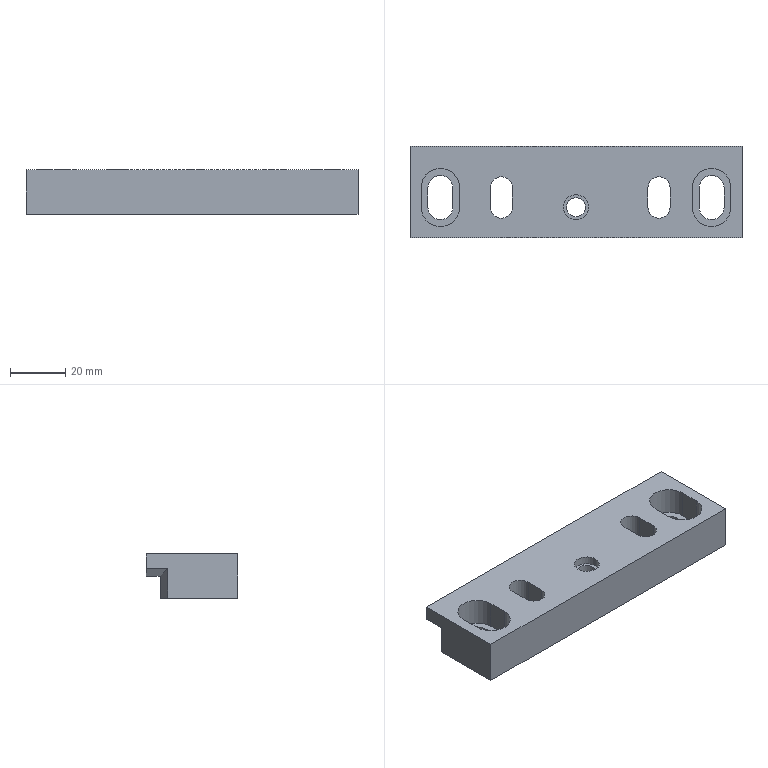Part | STEP file | lll_id4706_x_t | 1 solid | 41 faces | box 120 x 33 x 16 mm | volume 47542 mm3 | plane 27 | cylinder 14 | commonest cylinder face diameters 9 x5 8 x4 14 x4 6.8 x1
STEP:
#1=CARTESIAN_POINT('',(1165.435,-359.7,16.));
#2=VERTEX_POINT('',#1);
#3=CARTESIAN_POINT('',(1173.435,-359.7,16.));
#4=VERTEX_POINT('',#3);
#5=CARTESIAN_POINT('',(1169.435,-359.7,16.));
#6=DIRECTION('',(0.,0.,1.));
#7=DIRECTION('',(-1.,0.,0.));
#8=AXIS2_PLACEMENT_3D('',#5,#6,#7);
#9=CIRCLE('',#8,4.);
#10=EDGE_CURVE('',#2,#4,#9,.T.);
#11=ORIENTED_EDGE('',*,*,#10,.F.);
#12=CARTESIAN_POINT('',(1165.435,-352.7,16.));
#13=VERTEX_POINT('',#12);
#14=CARTESIAN_POINT('',(1165.435,-370.7,16.));
#15=DIRECTION('',(0.,-1.,0.));
#16=VECTOR('',#15,1.);
#17=LINE('',#14,#16);
#18=EDGE_CURVE('',#13,#2,#17,.T.);
#19=ORIENTED_EDGE('',*,*,#18,.F.);
#20=CARTESIAN_POINT('',(1173.435,-352.7,16.));
#21=VERTEX_POINT('',#20);
#22=CARTESIAN_POINT('',(1169.435,-352.7,16.));
#23=DIRECTION('',(0.,0.,1.));
#24=DIRECTION('',(-1.,0.,0.));
#25=AXIS2_PLACEMENT_3D('',#22,#23,#24);
#26=CIRCLE('',#25,4.);
#27=EDGE_CURVE('',#21,#13,#26,.T.);
#28=ORIENTED_EDGE('',*,*,#27,.F.);
#29=CARTESIAN_POINT('',(1173.435,-370.7,16.));
#30=DIRECTION('',(0.,1.,0.));
#31=VECTOR('',#30,1.);
#32=LINE('',#29,#31);
#33=EDGE_CURVE('',#4,#21,#32,.T.);
#34=ORIENTED_EDGE('',*,*,#33,.F.);
#35=EDGE_LOOP('',(#11,#19,#28,#34));
#36=FACE_BOUND('',#35,.T.);
#37=CARTESIAN_POINT('',(1108.435,-359.7,16.));
#38=VERTEX_POINT('',#37);
#39=CARTESIAN_POINT('',(1108.435,-352.7,16.));
#40=VERTEX_POINT('',#39);
#41=CARTESIAN_POINT('',(1108.435,-370.7,16.));
#42=DIRECTION('',(0.,1.,0.));
#43=VECTOR('',#42,1.);
#44=LINE('',#41,#43);
#45=EDGE_CURVE('',#38,#40,#44,.T.);
#46=ORIENTED_EDGE('',*,*,#45,.T.);
#47=CARTESIAN_POINT('',(1116.435,-352.7,16.));
#48=VERTEX_POINT('',#47);
#49=CARTESIAN_POINT('',(1112.435,-352.7,16.));
#50=DIRECTION('',(0.,0.,-1.));
#51=DIRECTION('',(-1.,0.,0.));
#52=AXIS2_PLACEMENT_3D('',#49,#50,#51);
#53=CIRCLE('',#52,4.);
#54=EDGE_CURVE('',#40,#48,#53,.T.);
#55=ORIENTED_EDGE('',*,*,#54,.T.);
#56=CARTESIAN_POINT('',(1116.435,-359.7,16.));
#57=VERTEX_POINT('',#56);
#58=CARTESIAN_POINT('',(1116.435,-370.7,16.));
#59=DIRECTION('',(0.,-1.,0.));
#60=VECTOR('',#59,1.);
#61=LINE('',#58,#60);
#62=EDGE_CURVE('',#48,#57,#61,.T.);
#63=ORIENTED_EDGE('',*,*,#62,.T.);
#64=CARTESIAN_POINT('',(1112.435,-359.7,16.));
#65=DIRECTION('',(0.,0.,-1.));
#66=DIRECTION('',(-1.,0.,0.));
#67=AXIS2_PLACEMENT_3D('',#64,#65,#66);
#68=CIRCLE('',#67,4.);
#69=EDGE_CURVE('',#57,#38,#68,.T.);
#70=ORIENTED_EDGE('',*,*,#69,.T.);
#71=EDGE_LOOP('',(#46,#55,#63,#70));
#72=FACE_BOUND('',#71,.T.);
#73=CARTESIAN_POINT('',(1079.435,-370.7,16.));
#74=VERTEX_POINT('',#73);
#75=CARTESIAN_POINT('',(1199.435,-370.7,16.));
#76=VERTEX_POINT('',#75);
#77=CARTESIAN_POINT('',(1079.435,-370.7,16.));
#78=DIRECTION('',(1.,0.,0.));
#79=VECTOR('',#78,1.);
#80=LINE('',#77,#79);
#81=EDGE_CURVE('',#74,#76,#80,.T.);
#82=ORIENTED_EDGE('',*,*,#81,.T.);
#83=CARTESIAN_POINT('',(1199.435,-337.7,16.));
#84=VERTEX_POINT('',#83);
#85=CARTESIAN_POINT('',(1199.435,-370.7,16.));
#86=DIRECTION('',(0.,1.,0.));
#87=VECTOR('',#86,1.);
#88=LINE('',#85,#87);
#89=EDGE_CURVE('',#76,#84,#88,.T.);
#90=ORIENTED_EDGE('',*,*,#89,.T.);
#91=CARTESIAN_POINT('',(1079.435,-337.7,16.));
#92=VERTEX_POINT('',#91);
#93=CARTESIAN_POINT('',(1159.435,-337.7,16.));
#94=DIRECTION('',(-1.,0.,0.));
#95=VECTOR('',#94,1.);
#96=LINE('',#93,#95);
#97=EDGE_CURVE('',#84,#92,#96,.T.);
#98=ORIENTED_EDGE('',*,*,#97,.T.);
#99=CARTESIAN_POINT('',(1079.435,-337.7,16.));
#100=DIRECTION('',(0.,-1.,0.));
#101=VECTOR('',#100,1.);
#102=LINE('',#99,#101);
#103=EDGE_CURVE('',#92,#74,#102,.T.);
#104=ORIENTED_EDGE('',*,*,#103,.T.);
#105=EDGE_LOOP('',(#82,#90,#98,#104));
#106=FACE_BOUND('',#105,.T.);
#107=CARTESIAN_POINT('',(1083.435,-359.7,16.));
#108=VERTEX_POINT('',#107);
#109=CARTESIAN_POINT('',(1097.435,-359.7,16.));
#110=VERTEX_POINT('',#109);
#111=CARTESIAN_POINT('',(1090.435,-359.7,16.));
#112=DIRECTION('',(0.,0.,1.));
#113=DIRECTION('',(-1.,0.,0.));
#114=AXIS2_PLACEMENT_3D('',#111,#112,#113);
#115=CIRCLE('',#114,7.);
#116=EDGE_CURVE('',#108,#110,#115,.T.);
#117=ORIENTED_EDGE('',*,*,#116,.F.);
#118=CARTESIAN_POINT('',(1083.435,-352.7,16.));
#119=VERTEX_POINT('',#118);
#120=CARTESIAN_POINT('',(1083.435,-370.7,16.));
#121=DIRECTION('',(0.,-1.,0.));
#122=VECTOR('',#121,1.);
#123=LINE('',#120,#122);
#124=EDGE_CURVE('',#119,#108,#123,.T.);
#125=ORIENTED_EDGE('',*,*,#124,.F.);
#126=CARTESIAN_POINT('',(1097.435,-352.7,16.));
#127=VERTEX_POINT('',#126);
#128=CARTESIAN_POINT('',(1090.435,-352.7,16.));
#129=DIRECTION('',(0.,0.,1.));
#130=DIRECTION('',(-1.,0.,0.));
#131=AXIS2_PLACEMENT_3D('',#128,#129,#130);
#132=CIRCLE('',#131,7.);
#133=EDGE_CURVE('',#127,#119,#132,.T.);
#134=ORIENTED_EDGE('',*,*,#133,.F.);
#135=CARTESIAN_POINT('',(1097.435,-370.7,16.));
#136=DIRECTION('',(0.,1.,0.));
#137=VECTOR('',#136,1.);
#138=LINE('',#135,#137);
#139=EDGE_CURVE('',#110,#127,#138,.T.);
#140=ORIENTED_EDGE('',*,*,#139,.F.);
#141=EDGE_LOOP('',(#117,#125,#134,#140));
#142=FACE_BOUND('',#141,.T.);
#143=CARTESIAN_POINT('',(1195.435,-352.7,16.));
#144=VERTEX_POINT('',#143);
#145=CARTESIAN_POINT('',(1181.435,-352.7,16.));
#146=VERTEX_POINT('',#145);
#147=CARTESIAN_POINT('',(1188.435,-352.7,16.));
#148=DIRECTION('',(0.,0.,1.));
#149=DIRECTION('',(-1.,0.,0.));
#150=AXIS2_PLACEMENT_3D('',#147,#148,#149);
#151=CIRCLE('',#150,7.);
#152=EDGE_CURVE('',#144,#146,#151,.T.);
#153=ORIENTED_EDGE('',*,*,#152,.F.);
#154=CARTESIAN_POINT('',(1195.435,-359.7,16.));
#155=VERTEX_POINT('',#154);
#156=CARTESIAN_POINT('',(1195.435,-370.7,16.));
#157=DIRECTION('',(0.,1.,0.));
#158=VECTOR('',#157,1.);
#159=LINE('',#156,#158);
#160=EDGE_CURVE('',#155,#144,#159,.T.);
#161=ORIENTED_EDGE('',*,*,#160,.F.);
#162=CARTESIAN_POINT('',(1181.435,-359.7,16.));
#163=VERTEX_POINT('',#162);
#164=CARTESIAN_POINT('',(1188.435,-359.7,16.));
#165=DIRECTION('',(0.,0.,1.));
#166=DIRECTION('',(-1.,0.,0.));
#167=AXIS2_PLACEMENT_3D('',#164,#165,#166);
#168=CIRCLE('',#167,7.);
#169=EDGE_CURVE('',#163,#155,#168,.T.);
#170=ORIENTED_EDGE('',*,*,#169,.F.);
#171=CARTESIAN_POINT('',(1181.435,-370.7,16.));
#172=DIRECTION('',(0.,-1.,0.));
#173=VECTOR('',#172,1.);
#174=LINE('',#171,#173);
#175=EDGE_CURVE('',#146,#163,#174,.T.);
#176=ORIENTED_EDGE('',*,*,#175,.F.);
#177=EDGE_LOOP('',(#153,#161,#170,#176));
#178=FACE_BOUND('',#177,.T.);
#179=CARTESIAN_POINT('',(1134.935,-359.7,16.));
#180=VERTEX_POINT('',#179);
#181=CARTESIAN_POINT('',(1139.435,-359.7,16.));
#182=DIRECTION('',(0.,0.,1.));
#183=DIRECTION('',(-1.,0.,0.));
#184=AXIS2_PLACEMENT_3D('',#181,#182,#183);
#185=CIRCLE('',#184,4.5);
#186=EDGE_CURVE('',#180,#180,#185,.T.);
#187=ORIENTED_EDGE('',*,*,#186,.F.);
#188=EDGE_LOOP('',(#187));
#189=FACE_BOUND('',#188,.T.);
#190=CARTESIAN_POINT('',(1159.435,-370.7,16.));
#191=DIRECTION('',(0.,0.,1.));
#192=DIRECTION('',(-1.,0.,0.));
#193=AXIS2_PLACEMENT_3D('',#190,#191,#192);
#194=PLANE('',#193);
#195=ADVANCED_FACE('',(#36,#72,#106,#142,#178,#189),#194,.T.);
#196=CARTESIAN_POINT('',(1094.935,-352.7,0.));
#197=VERTEX_POINT('',#196);
#198=CARTESIAN_POINT('',(1094.935,-359.7,0.));
#199=VERTEX_POINT('',#198);
#200=CARTESIAN_POINT('',(1094.935,-352.7,0.));
#201=DIRECTION('',(0.,-1.,0.));
#202=VECTOR('',#201,1.);
#203=LINE('',#200,#202);
#204=EDGE_CURVE('',#197,#199,#203,.T.);
#205=ORIENTED_EDGE('',*,*,#204,.F.);
#206=CARTESIAN_POINT('',(1085.935,-352.7,0.));
#207=VERTEX_POINT('',#206);
#208=CARTESIAN_POINT('',(1090.435,-352.7,0.));
#209=DIRECTION('',(0.,0.,-1.));
#210=DIRECTION('',(-1.,0.,0.));
#211=AXIS2_PLACEMENT_3D('',#208,#209,#210);
#212=CIRCLE('',#211,4.5);
#213=EDGE_CURVE('',#207,#197,#212,.T.);
#214=ORIENTED_EDGE('',*,*,#213,.F.);
#215=CARTESIAN_POINT('',(1085.935,-359.7,0.));
#216=VERTEX_POINT('',#215);
#217=CARTESIAN_POINT('',(1085.935,-359.7,0.));
#218=DIRECTION('',(0.,1.,0.));
#219=VECTOR('',#218,1.);
#220=LINE('',#217,#219);
#221=EDGE_CURVE('',#216,#207,#220,.T.);
#222=ORIENTED_EDGE('',*,*,#221,.F.);
#223=CARTESIAN_POINT('',(1090.435,-359.7,0.));
#224=DIRECTION('',(0.,0.,-1.));
#225=DIRECTION('',(-1.,0.,0.));
#226=AXIS2_PLACEMENT_3D('',#223,#224,#225);
#227=CIRCLE('',#226,4.5);
#228=EDGE_CURVE('',#199,#216,#227,.T.);
#229=ORIENTED_EDGE('',*,*,#228,.F.);
#230=EDGE_LOOP('',(#205,#214,#222,#229));
#231=FACE_BOUND('',#230,.T.);
#232=CARTESIAN_POINT('',(1183.935,-352.7,0.));
#233=VERTEX_POINT('',#232);
#234=CARTESIAN_POINT('',(1183.935,-359.7,0.));
#235=VERTEX_POINT('',#234);
#236=CARTESIAN_POINT('',(1183.935,-352.7,0.));
#237=DIRECTION('',(0.,-1.,0.));
#238=VECTOR('',#237,1.);
#239=LINE('',#236,#238);
#240=EDGE_CURVE('',#233,#235,#239,.T.);
#241=ORIENTED_EDGE('',*,*,#240,.T.);
#242=CARTESIAN_POINT('',(1192.935,-359.7,0.));
#243=VERTEX_POINT('',#242);
#244=CARTESIAN_POINT('',(1188.435,-359.7,0.));
#245=DIRECTION('',(0.,0.,1.));
#246=DIRECTION('',(-1.,0.,0.));
#247=AXIS2_PLACEMENT_3D('',#244,#245,#246);
#248=CIRCLE('',#247,4.5);
#249=EDGE_CURVE('',#235,#243,#248,.T.);
#250=ORIENTED_EDGE('',*,*,#249,.T.);
#251=CARTESIAN_POINT('',(1192.935,-352.7,0.));
#252=VERTEX_POINT('',#251);
#253=CARTESIAN_POINT('',(1192.935,-359.7,0.));
#254=DIRECTION('',(0.,1.,0.));
#255=VECTOR('',#254,1.);
#256=LINE('',#253,#255);
#257=EDGE_CURVE('',#243,#252,#256,.T.);
#258=ORIENTED_EDGE('',*,*,#257,.T.);
#259=CARTESIAN_POINT('',(1188.435,-352.7,0.));
#260=DIRECTION('',(0.,0.,1.));
#261=DIRECTION('',(-1.,0.,0.));
#262=AXIS2_PLACEMENT_3D('',#259,#260,#261);
#263=CIRCLE('',#262,4.5);
#264=EDGE_CURVE('',#252,#233,#263,.T.);
#265=ORIENTED_EDGE('',*,*,#264,.T.);
#266=EDGE_LOOP('',(#241,#250,#258,#265));
#267=FACE_BOUND('',#266,.T.);
#268=CARTESIAN_POINT('',(1199.435,-345.38,0.));
#269=VERTEX_POINT('',#268);
#270=CARTESIAN_POINT('',(1189.434,-342.7,0.));
#271=VERTEX_POINT('',#270);
#272=CARTESIAN_POINT('',(1199.435,-345.38,0.));
#273=DIRECTION('',(-0.9659,0.2588,0.));
#274=VECTOR('',#273,1.);
#275=LINE('',#272,#274);
#276=EDGE_CURVE('',#269,#271,#275,.T.);
#277=ORIENTED_EDGE('',*,*,#276,.F.);
#278=CARTESIAN_POINT('',(1199.435,-370.7,0.));
#279=VERTEX_POINT('',#278);
#280=CARTESIAN_POINT('',(1199.435,-370.7,0.));
#281=DIRECTION('',(0.,1.,0.));
#282=VECTOR('',#281,1.);
#283=LINE('',#280,#282);
#284=EDGE_CURVE('',#279,#269,#283,.T.);
#285=ORIENTED_EDGE('',*,*,#284,.F.);
#286=CARTESIAN_POINT('',(1079.435,-370.7,0.));
#287=VERTEX_POINT('',#286);
#288=CARTESIAN_POINT('',(1079.435,-370.7,0.));
#289=DIRECTION('',(1.,0.,0.));
#290=VECTOR('',#289,1.);
#291=LINE('',#288,#290);
#292=EDGE_CURVE('',#287,#279,#291,.T.);
#293=ORIENTED_EDGE('',*,*,#292,.F.);
#294=CARTESIAN_POINT('',(1079.435,-345.379,0.));
#295=VERTEX_POINT('',#294);
#296=CARTESIAN_POINT('',(1079.435,-337.7,0.));
#297=DIRECTION('',(0.,-1.,0.));
#298=VECTOR('',#297,1.);
#299=LINE('',#296,#298);
#300=EDGE_CURVE('',#295,#287,#299,.T.);
#301=ORIENTED_EDGE('',*,*,#300,.F.);
#302=CARTESIAN_POINT('',(1089.434,-342.7,0.));
#303=VERTEX_POINT('',#302);
#304=CARTESIAN_POINT('',(1089.434,-342.7,0.));
#305=DIRECTION('',(-0.9659,-0.2588,0.));
#306=VECTOR('',#305,1.);
#307=LINE('',#304,#306);
#308=EDGE_CURVE('',#303,#295,#307,.T.);
#309=ORIENTED_EDGE('',*,*,#308,.F.);
#310=CARTESIAN_POINT('',(1149.434,-342.7,0.));
#311=DIRECTION('',(-1.,0.,0.));
#312=VECTOR('',#311,1.);
#313=LINE('',#310,#312);
#314=EDGE_CURVE('',#271,#303,#313,.T.);
#315=ORIENTED_EDGE('',*,*,#314,.F.);
#316=EDGE_LOOP('',(#277,#285,#293,#301,#309,#315));
#317=FACE_BOUND('',#316,.T.);
#318=CARTESIAN_POINT('',(1116.435,-352.7,0.));
#319=VERTEX_POINT('',#318);
#320=CARTESIAN_POINT('',(1108.435,-352.7,0.));
#321=VERTEX_POINT('',#320);
#322=CARTESIAN_POINT('',(1112.435,-352.7,0.));
#323=DIRECTION('',(0.,0.,1.));
#324=DIRECTION('',(-1.,0.,0.));
#325=AXIS2_PLACEMENT_3D('',#322,#323,#324);
#326=CIRCLE('',#325,4.);
#327=EDGE_CURVE('',#319,#321,#326,.T.);
#328=ORIENTED_EDGE('',*,*,#327,.T.);
#329=CARTESIAN_POINT('',(1108.435,-359.7,0.));
#330=VERTEX_POINT('',#329);
#331=CARTESIAN_POINT('',(1108.435,-352.7,0.));
#332=DIRECTION('',(0.,-1.,0.));
#333=VECTOR('',#332,1.);
#334=LINE('',#331,#333);
#335=EDGE_CURVE('',#321,#330,#334,.T.);
#336=ORIENTED_EDGE('',*,*,#335,.T.);
#337=CARTESIAN_POINT('',(1116.435,-359.7,0.));
#338=VERTEX_POINT('',#337);
#339=CARTESIAN_POINT('',(1112.435,-359.7,0.));
#340=DIRECTION('',(0.,0.,1.));
#341=DIRECTION('',(-1.,0.,0.));
#342=AXIS2_PLACEMENT_3D('',#339,#340,#341);
#343=CIRCLE('',#342,4.);
#344=EDGE_CURVE('',#330,#338,#343,.T.);
#345=ORIENTED_EDGE('',*,*,#344,.T.);
#346=CARTESIAN_POINT('',(1116.435,-359.7,0.));
#347=DIRECTION('',(0.,1.,0.));
#348=VECTOR('',#347,1.);
#349=LINE('',#346,#348);
#350=EDGE_CURVE('',#338,#319,#349,.T.);
#351=ORIENTED_EDGE('',*,*,#350,.T.);
#352=EDGE_LOOP('',(#328,#336,#345,#351));
#353=FACE_BOUND('',#352,.T.);
#354=CARTESIAN_POINT('',(1165.435,-359.7,0.));
#355=VERTEX_POINT('',#354);
#356=CARTESIAN_POINT('',(1165.435,-352.7,0.));
#357=VERTEX_POINT('',#356);
#358=CARTESIAN_POINT('',(1165.435,-359.7,0.));
#359=DIRECTION('',(0.,1.,0.));
#360=VECTOR('',#359,1.);
#361=LINE('',#358,#360);
#362=EDGE_CURVE('',#355,#357,#361,.T.);
#363=ORIENTED_EDGE('',*,*,#362,.F.);
#364=CARTESIAN_POINT('',(1173.435,-359.7,0.));
#365=VERTEX_POINT('',#364);
#366=CARTESIAN_POINT('',(1169.435,-359.7,0.));
#367=DIRECTION('',(0.,0.,-1.));
#368=DIRECTION('',(-1.,0.,0.));
#369=AXIS2_PLACEMENT_3D('',#366,#367,#368);
#370=CIRCLE('',#369,4.);
#371=EDGE_CURVE('',#365,#355,#370,.T.);
#372=ORIENTED_EDGE('',*,*,#371,.F.);
#373=CARTESIAN_POINT('',(1173.435,-352.7,0.));
#374=VERTEX_POINT('',#373);
#375=CARTESIAN_POINT('',(1173.435,-352.7,0.));
#376=DIRECTION('',(0.,-1.,0.));
#377=VECTOR('',#376,1.);
#378=LINE('',#375,#377);
#379=EDGE_CURVE('',#374,#365,#378,.T.);
#380=ORIENTED_EDGE('',*,*,#379,.F.);
#381=CARTESIAN_POINT('',(1169.435,-352.7,0.));
#382=DIRECTION('',(0.,0.,-1.));
#383=DIRECTION('',(-1.,0.,0.));
#384=AXIS2_PLACEMENT_3D('',#381,#382,#383);
#385=CIRCLE('',#384,4.);
#386=EDGE_CURVE('',#357,#374,#385,.T.);
#387=ORIENTED_EDGE('',*,*,#386,.F.);
#388=EDGE_LOOP('',(#363,#372,#380,#387));
#389=FACE_BOUND('',#388,.T.);
#390=CARTESIAN_POINT('',(1136.035,-359.7,0.));
#391=VERTEX_POINT('',#390);
#392=CARTESIAN_POINT('',(1139.435,-359.7,0.));
#393=DIRECTION('',(0.,0.,1.));
#394=DIRECTION('',(-1.,0.,0.));
#395=AXIS2_PLACEMENT_3D('',#392,#393,#394);
#396=CIRCLE('',#395,3.4);
#397=EDGE_CURVE('',#391,#391,#396,.T.);
#398=ORIENTED_EDGE('',*,*,#397,.T.);
#399=EDGE_LOOP('',(#398));
#400=FACE_BOUND('',#399,.T.);
#401=CARTESIAN_POINT('',(1159.435,-370.7,0.));
#402=DIRECTION('',(0.,0.,1.));
#403=DIRECTION('',(-1.,0.,0.));
#404=AXIS2_PLACEMENT_3D('',#401,#402,#403);
#405=PLANE('',#404);
#406=ADVANCED_FACE('',(#231,#267,#317,#353,#389,#400),#405,.F.);
#407=CARTESIAN_POINT('',(1199.435,-337.7,10.679));
#408=VERTEX_POINT('',#407);
#409=CARTESIAN_POINT('',(1199.435,-337.7,16.));
#410=DIRECTION('',(0.,0.,-1.));
#411=VECTOR('',#410,1.);
#412=LINE('',#409,#411);
#413=EDGE_CURVE('',#84,#408,#412,.T.);
#414=ORIENTED_EDGE('',*,*,#413,.T.);
#415=CARTESIAN_POINT('',(1189.435,-337.7,8.));
#416=VERTEX_POINT('',#415);
#417=CARTESIAN_POINT('',(1189.435,-337.7,8.));
#418=DIRECTION('',(-0.9659,0.,-0.2588));
#419=VECTOR('',#418,1.);
#420=LINE('',#417,#419);
#421=EDGE_CURVE('',#408,#416,#420,.T.);
#422=ORIENTED_EDGE('',*,*,#421,.T.);
#423=CARTESIAN_POINT('',(1089.435,-337.7,8.));
#424=VERTEX_POINT('',#423);
#425=CARTESIAN_POINT('',(1159.435,-337.7,8.));
#426=DIRECTION('',(1.,0.,0.));
#427=VECTOR('',#426,1.);
#428=LINE('',#425,#427);
#429=EDGE_CURVE('',#424,#416,#428,.T.);
#430=ORIENTED_EDGE('',*,*,#429,.F.);
#431=CARTESIAN_POINT('',(1079.435,-337.7,10.679));
#432=VERTEX_POINT('',#431);
#433=CARTESIAN_POINT('',(1089.435,-337.7,8.));
#434=DIRECTION('',(-0.9659,0.,0.2588));
#435=VECTOR('',#434,1.);
#436=LINE('',#433,#435);
#437=EDGE_CURVE('',#424,#432,#436,.T.);
#438=ORIENTED_EDGE('',*,*,#437,.T.);
#439=CARTESIAN_POINT('',(1079.435,-337.7,16.));
#440=DIRECTION('',(0.,0.,-1.));
#441=VECTOR('',#440,1.);
#442=LINE('',#439,#441);
#443=EDGE_CURVE('',#92,#432,#442,.T.);
#444=ORIENTED_EDGE('',*,*,#443,.F.);
#445=ORIENTED_EDGE('',*,*,#97,.F.);
#446=EDGE_LOOP('',(#414,#422,#430,#438,#444,#445));
#447=FACE_OUTER_BOUND('',#446,.T.);
#448=CARTESIAN_POINT('',(1159.435,-337.7,16.));
#449=DIRECTION('',(0.,-1.,0.));
#450=DIRECTION('',(0.,0.,1.));
#451=AXIS2_PLACEMENT_3D('',#448,#449,#450);
#452=PLANE('',#451);
#453=ADVANCED_FACE('',(#447),#452,.F.);
#454=ORIENTED_EDGE('',*,*,#292,.T.);
#455=CARTESIAN_POINT('',(1199.435,-370.7,16.));
#456=DIRECTION('',(0.,0.,-1.));
#457=VECTOR('',#456,1.);
#458=LINE('',#455,#457);
#459=EDGE_CURVE('',#76,#279,#458,.T.);
#460=ORIENTED_EDGE('',*,*,#459,.F.);
#461=ORIENTED_EDGE('',*,*,#81,.F.);
#462=CARTESIAN_POINT('',(1079.435,-370.7,16.));
#463=DIRECTION('',(0.,0.,-1.));
#464=VECTOR('',#463,1.);
#465=LINE('',#462,#464);
#466=EDGE_CURVE('',#74,#287,#465,.T.);
#467=ORIENTED_EDGE('',*,*,#466,.T.);
#468=EDGE_LOOP('',(#454,#460,#461,#467));
#469=FACE_OUTER_BOUND('',#468,.T.);
#470=CARTESIAN_POINT('',(1079.435,-370.7,16.));
#471=DIRECTION('',(0.,1.,0.));
#472=DIRECTION('',(0.,0.,-1.));
#473=AXIS2_PLACEMENT_3D('',#470,#471,#472);
#474=PLANE('',#473);
#475=ADVANCED_FACE('',(#469),#474,.F.);
#476=CARTESIAN_POINT('',(1199.435,-345.38,10.679));
#477=VERTEX_POINT('',#476);
#478=CARTESIAN_POINT('',(1199.435,-345.38,8.));
#479=DIRECTION('',(0.,0.,-1.));
#480=VECTOR('',#479,1.);
#481=LINE('',#478,#480);
#482=EDGE_CURVE('',#477,#269,#481,.T.);
#483=ORIENTED_EDGE('',*,*,#482,.F.);
#484=CARTESIAN_POINT('',(1199.435,-337.7,10.679));
#485=DIRECTION('',(0.,1.,0.));
#486=VECTOR('',#485,1.);
#487=LINE('',#484,#486);
#488=EDGE_CURVE('',#477,#408,#487,.T.);
#489=ORIENTED_EDGE('',*,*,#488,.T.);
#490=ORIENTED_EDGE('',*,*,#413,.F.);
#491=ORIENTED_EDGE('',*,*,#89,.F.);
#492=ORIENTED_EDGE('',*,*,#459,.T.);
#493=ORIENTED_EDGE('',*,*,#284,.T.);
#494=EDGE_LOOP('',(#483,#489,#490,#491,#492,#493));
#495=FACE_OUTER_BOUND('',#494,.T.);
#496=CARTESIAN_POINT('',(1199.435,-370.7,16.));
#497=DIRECTION('',(-1.,0.,0.));
#498=DIRECTION('',(0.,0.,-1.));
#499=AXIS2_PLACEMENT_3D('',#496,#497,#498);
#500=PLANE('',#499);
#501=ADVANCED_FACE('',(#495),#500,.F.);
#502=ORIENTED_EDGE('',*,*,#443,.T.);
#503=CARTESIAN_POINT('',(1079.435,-345.379,10.679));
#504=VERTEX_POINT('',#503);
#505=CARTESIAN_POINT('',(1079.435,-345.379,10.679));
#506=DIRECTION('',(0.,-1.,0.));
#507=VECTOR('',#506,1.);
#508=LINE('',#505,#507);
#509=EDGE_CURVE('',#432,#504,#508,.T.);
#510=ORIENTED_EDGE('',*,*,#509,.T.);
#511=CARTESIAN_POINT('',(1079.435,-345.379,8.));
#512=DIRECTION('',(0.,0.,-1.));
#513=VECTOR('',#512,1.);
#514=LINE('',#511,#513);
#515=EDGE_CURVE('',#504,#295,#514,.T.);
#516=ORIENTED_EDGE('',*,*,#515,.T.);
#517=ORIENTED_EDGE('',*,*,#300,.T.);
#518=ORIENTED_EDGE('',*,*,#466,.F.);
#519=ORIENTED_EDGE('',*,*,#103,.F.);
#520=EDGE_LOOP('',(#502,#510,#516,#517,#518,#519));
#521=FACE_OUTER_BOUND('',#520,.T.);
#522=CARTESIAN_POINT('',(1079.435,-337.7,16.));
#523=DIRECTION('',(1.,0.,0.));
#524=DIRECTION('',(0.,0.,1.));
#525=AXIS2_PLACEMENT_3D('',#522,#523,#524);
#526=PLANE('',#525);
#527=ADVANCED_FACE('',(#521),#526,.F.);
#528=ORIENTED_EDGE('',*,*,#429,.T.);
#529=CARTESIAN_POINT('',(1189.435,-342.701,8.));
#530=VERTEX_POINT('',#529);
#531=CARTESIAN_POINT('',(1189.435,-345.38,8.));
#532=DIRECTION('',(0.,-1.,0.));
#533=VECTOR('',#532,1.);
#534=LINE('',#531,#533);
#535=EDGE_CURVE('',#416,#530,#534,.T.);
#536=ORIENTED_EDGE('',*,*,#535,.T.);
#537=CARTESIAN_POINT('',(1189.434,-342.7,8.));
#538=VERTEX_POINT('',#537);
#539=CARTESIAN_POINT('',(1199.435,-345.38,8.));
#540=DIRECTION('',(0.9659,-0.2588,0.));
#541=VECTOR('',#540,1.);
#542=LINE('',#539,#541);
#543=EDGE_CURVE('',#538,#530,#542,.T.);
#544=ORIENTED_EDGE('',*,*,#543,.F.);
#545=CARTESIAN_POINT('',(1089.435,-342.7,8.));
#546=VERTEX_POINT('',#545);
#547=CARTESIAN_POINT('',(1149.434,-342.7,8.));
#548=DIRECTION('',(1.,0.,0.));
#549=VECTOR('',#548,1.);
#550=LINE('',#547,#549);
#551=EDGE_CURVE('',#546,#538,#550,.T.);
#552=ORIENTED_EDGE('',*,*,#551,.F.);
#553=CARTESIAN_POINT('',(1089.435,-337.7,8.));
#554=DIRECTION('',(0.,1.,0.));
#555=VECTOR('',#554,1.);
#556=LINE('',#553,#555);
#557=EDGE_CURVE('',#546,#424,#556,.T.);
#558=ORIENTED_EDGE('',*,*,#557,.T.);
#559=EDGE_LOOP('',(#528,#536,#544,#552,#558));
#560=FACE_OUTER_BOUND('',#559,.T.);
#561=CARTESIAN_POINT('',(1181.706,-317.091,8.));
#562=DIRECTION('',(0.,0.,-1.));
#563=DIRECTION('',(1.,0.,0.));
#564=AXIS2_PLACEMENT_3D('',#561,#562,#563);
#565=PLANE('',#564);
#566=ADVANCED_FACE('',(#560),#565,.T.);
#567=ORIENTED_EDGE('',*,*,#276,.T.);
#568=CARTESIAN_POINT('',(1189.434,-342.7,8.));
#569=DIRECTION('',(0.,0.,1.));
#570=VECTOR('',#569,1.);
#571=LINE('',#568,#570);
#572=EDGE_CURVE('',#271,#538,#571,.T.);
#573=ORIENTED_EDGE('',*,*,#572,.T.);
#574=ORIENTED_EDGE('',*,*,#543,.T.);
#575=CARTESIAN_POINT('',(1198.807,-345.212,10.511));
#576=DIRECTION('',(0.9351,-0.2506,0.2506));
#577=VECTOR('',#576,1.);
#578=LINE('',#575,#577);
#579=EDGE_CURVE('',#530,#477,#578,.T.);
#580=ORIENTED_EDGE('',*,*,#579,.T.);
#581=ORIENTED_EDGE('',*,*,#482,.T.);
#582=EDGE_LOOP('',(#567,#573,#574,#580,#581));
#583=FACE_OUTER_BOUND('',#582,.T.);
#584=CARTESIAN_POINT('',(1199.435,-345.38,8.));
#585=DIRECTION('',(-0.2588,-0.9659,0.));
#586=DIRECTION('',(0.9659,-0.2588,0.));
#587=AXIS2_PLACEMENT_3D('',#584,#585,#586);
#588=PLANE('',#587);
#589=ADVANCED_FACE('',(#583),#588,.F.);
#590=ORIENTED_EDGE('',*,*,#314,.T.);
#591=CARTESIAN_POINT('',(1089.434,-342.7,8.));
#592=VERTEX_POINT('',#591);
#593=CARTESIAN_POINT('',(1089.434,-342.7,8.));
#594=DIRECTION('',(0.,0.,1.));
#595=VECTOR('',#594,1.);
#596=LINE('',#593,#595);
#597=EDGE_CURVE('',#303,#592,#596,.T.);
#598=ORIENTED_EDGE('',*,*,#597,.T.);
#599=CARTESIAN_POINT('',(1145.414,-342.7,-7.));
#600=DIRECTION('',(0.9659,0.,-0.2588));
#601=VECTOR('',#600,1.);
#602=LINE('',#599,#601);
#603=EDGE_CURVE('',#592,#546,#602,.T.);
#604=ORIENTED_EDGE('',*,*,#603,.T.);
#605=ORIENTED_EDGE('',*,*,#551,.T.);
#606=ORIENTED_EDGE('',*,*,#572,.F.);
#607=EDGE_LOOP('',(#590,#598,#604,#605,#606));
#608=FACE_OUTER_BOUND('',#607,.T.);
#609=CARTESIAN_POINT('',(1149.434,-342.7,8.));
#610=DIRECTION('',(0.,-1.,0.));
#611=DIRECTION('',(0.,0.,1.));
#612=AXIS2_PLACEMENT_3D('',#609,#610,#611);
#613=PLANE('',#612);
#614=ADVANCED_FACE('',(#608),#613,.F.);
#615=ORIENTED_EDGE('',*,*,#308,.T.);
#616=ORIENTED_EDGE('',*,*,#515,.F.);
#617=CARTESIAN_POINT('',(1089.434,-342.7,8.));
#618=DIRECTION('',(0.9351,0.2506,-0.2506));
#619=VECTOR('',#618,1.);
#620=LINE('',#617,#619);
#621=EDGE_CURVE('',#504,#592,#620,.T.);
#622=ORIENTED_EDGE('',*,*,#621,.T.);
#623=ORIENTED_EDGE('',*,*,#597,.F.);
#624=EDGE_LOOP('',(#615,#616,#622,#623));
#625=FACE_OUTER_BOUND('',#624,.T.);
#626=CARTESIAN_POINT('',(1089.434,-342.7,8.));
#627=DIRECTION('',(0.2588,-0.9659,0.));
#628=DIRECTION('',(0.9659,0.2588,0.));
#629=AXIS2_PLACEMENT_3D('',#626,#627,#628);
#630=PLANE('',#629);
#631=ADVANCED_FACE('',(#625),#630,.F.);
#632=CARTESIAN_POINT('',(1108.435,-352.7,47.));
#633=DIRECTION('',(0.,0.,1.));
#634=VECTOR('',#633,1.);
#635=LINE('',#632,#634);
#636=EDGE_CURVE('',#321,#40,#635,.T.);
#637=ORIENTED_EDGE('',*,*,#636,.F.);
#638=ORIENTED_EDGE('',*,*,#327,.F.);
#639=CARTESIAN_POINT('',(1116.435,-352.7,47.));
#640=DIRECTION('',(0.,0.,1.));
#641=VECTOR('',#640,1.);
#642=LINE('',#639,#641);
#643=EDGE_CURVE('',#319,#48,#642,.T.);
#644=ORIENTED_EDGE('',*,*,#643,.T.);
#645=ORIENTED_EDGE('',*,*,#54,.F.);
#646=EDGE_LOOP('',(#637,#638,#644,#645));
#647=FACE_OUTER_BOUND('',#646,.T.);
#648=CARTESIAN_POINT('',(1112.435,-352.7,47.));
#649=DIRECTION('',(0.,0.,-1.));
#650=DIRECTION('',(1.,0.,0.));
#651=AXIS2_PLACEMENT_3D('',#648,#649,#650);
#652=CYLINDRICAL_SURFACE('',#651,4.);
#653=ADVANCED_FACE('',(#647),#652,.F.);
#654=CARTESIAN_POINT('',(1108.435,-359.7,47.));
#655=DIRECTION('',(0.,0.,1.));
#656=VECTOR('',#655,1.);
#657=LINE('',#654,#656);
#658=EDGE_CURVE('',#330,#38,#657,.T.);
#659=ORIENTED_EDGE('',*,*,#658,.F.);
#660=ORIENTED_EDGE('',*,*,#335,.F.);
#661=ORIENTED_EDGE('',*,*,#636,.T.);
#662=ORIENTED_EDGE('',*,*,#45,.F.);
#663=EDGE_LOOP('',(#659,#660,#661,#662));
#664=FACE_OUTER_BOUND('',#663,.T.);
#665=CARTESIAN_POINT('',(1108.435,-352.7,47.));
#666=DIRECTION('',(1.,0.,0.));
#667=DIRECTION('',(0.,0.,1.));
#668=AXIS2_PLACEMENT_3D('',#665,#666,#667);
#669=PLANE('',#668);
#670=ADVANCED_FACE('',(#664),#669,.T.);
#671=CARTESIAN_POINT('',(1116.435,-359.7,47.));
#672=DIRECTION('',(0.,0.,1.));
#673=VECTOR('',#672,1.);
#674=LINE('',#671,#673);
#675=EDGE_CURVE('',#338,#57,#674,.T.);
#676=ORIENTED_EDGE('',*,*,#675,.F.);
#677=ORIENTED_EDGE('',*,*,#344,.F.);
#678=ORIENTED_EDGE('',*,*,#658,.T.);
#679=ORIENTED_EDGE('',*,*,#69,.F.);
#680=EDGE_LOOP('',(#676,#677,#678,#679));
#681=FACE_OUTER_BOUND('',#680,.T.);
#682=CARTESIAN_POINT('',(1112.435,-359.7,47.));
#683=DIRECTION('',(0.,0.,-1.));
#684=DIRECTION('',(1.,0.,0.));
#685=AXIS2_PLACEMENT_3D('',#682,#683,#684);
#686=CYLINDRICAL_SURFACE('',#685,4.);
#687=ADVANCED_FACE('',(#681),#686,.F.);
#688=ORIENTED_EDGE('',*,*,#643,.F.);
#689=ORIENTED_EDGE('',*,*,#350,.F.);
#690=ORIENTED_EDGE('',*,*,#675,.T.);
#691=ORIENTED_EDGE('',*,*,#62,.F.);
#692=EDGE_LOOP('',(#688,#689,#690,#691));
#693=FACE_OUTER_BOUND('',#692,.T.);
#694=CARTESIAN_POINT('',(1116.435,-359.7,47.));
#695=DIRECTION('',(-1.,0.,0.));
#696=DIRECTION('',(0.,0.,-1.));
#697=AXIS2_PLACEMENT_3D('',#694,#695,#696);
#698=PLANE('',#697);
#699=ADVANCED_FACE('',(#693),#698,.T.);
#700=CARTESIAN_POINT('',(1183.935,-359.7,6.));
#701=VERTEX_POINT('',#700);
#702=CARTESIAN_POINT('',(1183.935,-352.7,6.));
#703=VERTEX_POINT('',#702);
#704=CARTESIAN_POINT('',(1183.935,-352.7,6.));
#705=DIRECTION('',(0.,1.,0.));
#706=VECTOR('',#705,1.);
#707=LINE('',#704,#706);
#708=EDGE_CURVE('',#701,#703,#707,.T.);
#709=ORIENTED_EDGE('',*,*,#708,.F.);
#710=CARTESIAN_POINT('',(1183.935,-359.7,47.));
#711=DIRECTION('',(0.,0.,1.));
#712=VECTOR('',#711,1.);
#713=LINE('',#710,#712);
#714=EDGE_CURVE('',#235,#701,#713,.T.);
#715=ORIENTED_EDGE('',*,*,#714,.F.);
#716=ORIENTED_EDGE('',*,*,#240,.F.);
#717=CARTESIAN_POINT('',(1183.935,-352.7,47.));
#718=DIRECTION('',(0.,0.,1.));
#719=VECTOR('',#718,1.);
#720=LINE('',#717,#719);
#721=EDGE_CURVE('',#233,#703,#720,.T.);
#722=ORIENTED_EDGE('',*,*,#721,.T.);
#723=EDGE_LOOP('',(#709,#715,#716,#722));
#724=FACE_OUTER_BOUND('',#723,.T.);
#725=CARTESIAN_POINT('',(1183.935,-352.7,47.));
#726=DIRECTION('',(1.,0.,0.));
#727=DIRECTION('',(0.,0.,1.));
#728=AXIS2_PLACEMENT_3D('',#725,#726,#727);
#729=PLANE('',#728);
#730=ADVANCED_FACE('',(#724),#729,.T.);
#731=CARTESIAN_POINT('',(1192.935,-359.7,6.));
#732=VERTEX_POINT('',#731);
#733=CARTESIAN_POINT('',(1188.435,-359.7,6.));
#734=DIRECTION('',(0.,0.,-1.));
#735=DIRECTION('',(1.,0.,0.));
#736=AXIS2_PLACEMENT_3D('',#733,#734,#735);
#737=CIRCLE('',#736,4.5);
#738=EDGE_CURVE('',#732,#701,#737,.T.);
#739=ORIENTED_EDGE('',*,*,#738,.F.);
#740=CARTESIAN_POINT('',(1192.935,-359.7,47.));
#741=DIRECTION('',(0.,0.,1.));
#742=VECTOR('',#741,1.);
#743=LINE('',#740,#742);
#744=EDGE_CURVE('',#243,#732,#743,.T.);
#745=ORIENTED_EDGE('',*,*,#744,.F.);
#746=ORIENTED_EDGE('',*,*,#249,.F.);
#747=ORIENTED_EDGE('',*,*,#714,.T.);
#748=EDGE_LOOP('',(#739,#745,#746,#747));
#749=FACE_OUTER_BOUND('',#748,.T.);
#750=CARTESIAN_POINT('',(1188.435,-359.7,47.));
#751=DIRECTION('',(0.,0.,-1.));
#752=DIRECTION('',(1.,0.,0.));
#753=AXIS2_PLACEMENT_3D('',#750,#751,#752);
#754=CYLINDRICAL_SURFACE('',#753,4.5);
#755=ADVANCED_FACE('',(#749),#754,.F.);
#756=CARTESIAN_POINT('',(1192.935,-352.7,6.));
#757=VERTEX_POINT('',#756);
#758=CARTESIAN_POINT('',(1192.935,-359.7,6.));
#759=DIRECTION('',(0.,-1.,0.));
#760=VECTOR('',#759,1.);
#761=LINE('',#758,#760);
#762=EDGE_CURVE('',#757,#732,#761,.T.);
#763=ORIENTED_EDGE('',*,*,#762,.F.);
#764=CARTESIAN_POINT('',(1192.935,-352.7,47.));
#765=DIRECTION('',(0.,0.,1.));
#766=VECTOR('',#765,1.);
#767=LINE('',#764,#766);
#768=EDGE_CURVE('',#252,#757,#767,.T.);
#769=ORIENTED_EDGE('',*,*,#768,.F.);
#770=ORIENTED_EDGE('',*,*,#257,.F.);
#771=ORIENTED_EDGE('',*,*,#744,.T.);
#772=EDGE_LOOP('',(#763,#769,#770,#771));
#773=FACE_OUTER_BOUND('',#772,.T.);
#774=CARTESIAN_POINT('',(1192.935,-359.7,47.));
#775=DIRECTION('',(-1.,0.,0.));
#776=DIRECTION('',(0.,0.,-1.));
#777=AXIS2_PLACEMENT_3D('',#774,#775,#776);
#778=PLANE('',#777);
#779=ADVANCED_FACE('',(#773),#778,.T.);
#780=CARTESIAN_POINT('',(1188.435,-352.7,6.));
#781=DIRECTION('',(0.,0.,-1.));
#782=DIRECTION('',(1.,0.,0.));
#783=AXIS2_PLACEMENT_3D('',#780,#781,#782);
#784=CIRCLE('',#783,4.5);
#785=EDGE_CURVE('',#703,#757,#784,.T.);
#786=ORIENTED_EDGE('',*,*,#785,.F.);
#787=ORIENTED_EDGE('',*,*,#721,.F.);
#788=ORIENTED_EDGE('',*,*,#264,.F.);
#789=ORIENTED_EDGE('',*,*,#768,.T.);
#790=EDGE_LOOP('',(#786,#787,#788,#789));
#791=FACE_OUTER_BOUND('',#790,.T.);
#792=CARTESIAN_POINT('',(1188.435,-352.7,47.));
#793=DIRECTION('',(0.,0.,-1.));
#794=DIRECTION('',(1.,0.,0.));
#795=AXIS2_PLACEMENT_3D('',#792,#793,#794);
#796=CYLINDRICAL_SURFACE('',#795,4.5);
#797=ADVANCED_FACE('',(#791),#796,.F.);
#798=ORIENTED_EDGE('',*,*,#10,.T.);
#799=CARTESIAN_POINT('',(1173.435,-359.7,47.));
#800=DIRECTION('',(0.,0.,1.));
#801=VECTOR('',#800,1.);
#802=LINE('',#799,#801);
#803=EDGE_CURVE('',#365,#4,#802,.T.);
#804=ORIENTED_EDGE('',*,*,#803,.F.);
#805=ORIENTED_EDGE('',*,*,#371,.T.);
#806=CARTESIAN_POINT('',(1165.435,-359.7,47.));
#807=DIRECTION('',(0.,0.,1.));
#808=VECTOR('',#807,1.);
#809=LINE('',#806,#808);
#810=EDGE_CURVE('',#355,#2,#809,.T.);
#811=ORIENTED_EDGE('',*,*,#810,.T.);
#812=EDGE_LOOP('',(#798,#804,#805,#811));
#813=FACE_OUTER_BOUND('',#812,.T.);
#814=CARTESIAN_POINT('',(1169.435,-359.7,47.));
#815=DIRECTION('',(0.,0.,-1.));
#816=DIRECTION('',(1.,0.,0.));
#817=AXIS2_PLACEMENT_3D('',#814,#815,#816);
#818=CYLINDRICAL_SURFACE('',#817,4.);
#819=ADVANCED_FACE('',(#813),#818,.F.);
#820=ORIENTED_EDGE('',*,*,#18,.T.);
#821=ORIENTED_EDGE('',*,*,#810,.F.);
#822=ORIENTED_EDGE('',*,*,#362,.T.);
#823=CARTESIAN_POINT('',(1165.435,-352.7,47.));
#824=DIRECTION('',(0.,0.,1.));
#825=VECTOR('',#824,1.);
#826=LINE('',#823,#825);
#827=EDGE_CURVE('',#357,#13,#826,.T.);
#828=ORIENTED_EDGE('',*,*,#827,.T.);
#829=EDGE_LOOP('',(#820,#821,#822,#828));
#830=FACE_OUTER_BOUND('',#829,.T.);
#831=CARTESIAN_POINT('',(1165.435,-359.7,47.));
#832=DIRECTION('',(-1.,0.,0.));
#833=DIRECTION('',(0.,0.,-1.));
#834=AXIS2_PLACEMENT_3D('',#831,#832,#833);
#835=PLANE('',#834);
#836=ADVANCED_FACE('',(#830),#835,.F.);
#837=ORIENTED_EDGE('',*,*,#27,.T.);
#838=ORIENTED_EDGE('',*,*,#827,.F.);
#839=ORIENTED_EDGE('',*,*,#386,.T.);
#840=CARTESIAN_POINT('',(1173.435,-352.7,47.));
#841=DIRECTION('',(0.,0.,1.));
#842=VECTOR('',#841,1.);
#843=LINE('',#840,#842);
#844=EDGE_CURVE('',#374,#21,#843,.T.);
#845=ORIENTED_EDGE('',*,*,#844,.T.);
#846=EDGE_LOOP('',(#837,#838,#839,#845));
#847=FACE_OUTER_BOUND('',#846,.T.);
#848=CARTESIAN_POINT('',(1169.435,-352.7,47.));
#849=DIRECTION('',(0.,0.,-1.));
#850=DIRECTION('',(1.,0.,0.));
#851=AXIS2_PLACEMENT_3D('',#848,#849,#850);
#852=CYLINDRICAL_SURFACE('',#851,4.);
#853=ADVANCED_FACE('',(#847),#852,.F.);
#854=ORIENTED_EDGE('',*,*,#33,.T.);
#855=ORIENTED_EDGE('',*,*,#844,.F.);
#856=ORIENTED_EDGE('',*,*,#379,.T.);
#857=ORIENTED_EDGE('',*,*,#803,.T.);
#858=EDGE_LOOP('',(#854,#855,#856,#857));
#859=FACE_OUTER_BOUND('',#858,.T.);
#860=CARTESIAN_POINT('',(1173.435,-352.7,47.));
#861=DIRECTION('',(1.,0.,0.));
#862=DIRECTION('',(0.,0.,1.));
#863=AXIS2_PLACEMENT_3D('',#860,#861,#862);
#864=PLANE('',#863);
#865=ADVANCED_FACE('',(#859),#864,.F.);
#866=CARTESIAN_POINT('',(1142.835,-359.7,13.));
#867=VERTEX_POINT('',#866);
#868=CARTESIAN_POINT('',(1139.435,-359.7,13.));
#869=DIRECTION('',(0.,0.,-1.));
#870=DIRECTION('',(1.,0.,0.));
#871=AXIS2_PLACEMENT_3D('',#868,#869,#870);
#872=CIRCLE('',#871,3.4);
#873=EDGE_CURVE('',#867,#867,#872,.T.);
#874=ORIENTED_EDGE('',*,*,#873,.F.);
#875=EDGE_LOOP('',(#874));
#876=FACE_BOUND('',#875,.T.);
#877=ORIENTED_EDGE('',*,*,#397,.F.);
#878=EDGE_LOOP('',(#877));
#879=FACE_BOUND('',#878,.T.);
#880=CARTESIAN_POINT('',(1139.435,-359.7,47.));
#881=DIRECTION('',(0.,0.,-1.));
#882=DIRECTION('',(1.,0.,0.));
#883=AXIS2_PLACEMENT_3D('',#880,#881,#882);
#884=CYLINDRICAL_SURFACE('',#883,3.4);
#885=ADVANCED_FACE('',(#876,#879),#884,.F.);
#886=CARTESIAN_POINT('',(1094.935,-352.7,6.));
#887=VERTEX_POINT('',#886);
#888=CARTESIAN_POINT('',(1094.935,-352.7,47.));
#889=DIRECTION('',(0.,0.,1.));
#890=VECTOR('',#889,1.);
#891=LINE('',#888,#890);
#892=EDGE_CURVE('',#197,#887,#891,.T.);
#893=ORIENTED_EDGE('',*,*,#892,.T.);
#894=CARTESIAN_POINT('',(1085.935,-352.7,6.));
#895=VERTEX_POINT('',#894);
#896=CARTESIAN_POINT('',(1090.435,-352.7,6.));
#897=DIRECTION('',(0.,0.,1.));
#898=DIRECTION('',(1.,0.,0.));
#899=AXIS2_PLACEMENT_3D('',#896,#897,#898);
#900=CIRCLE('',#899,4.5);
#901=EDGE_CURVE('',#887,#895,#900,.T.);
#902=ORIENTED_EDGE('',*,*,#901,.T.);
#903=CARTESIAN_POINT('',(1085.935,-352.7,47.));
#904=DIRECTION('',(0.,0.,1.));
#905=VECTOR('',#904,1.);
#906=LINE('',#903,#905);
#907=EDGE_CURVE('',#207,#895,#906,.T.);
#908=ORIENTED_EDGE('',*,*,#907,.F.);
#909=ORIENTED_EDGE('',*,*,#213,.T.);
#910=EDGE_LOOP('',(#893,#902,#908,#909));
#911=FACE_OUTER_BOUND('',#910,.T.);
#912=CARTESIAN_POINT('',(1090.435,-352.7,47.));
#913=DIRECTION('',(0.,0.,-1.));
#914=DIRECTION('',(1.,0.,0.));
#915=AXIS2_PLACEMENT_3D('',#912,#913,#914);
#916=CYLINDRICAL_SURFACE('',#915,4.5);
#917=ADVANCED_FACE('',(#911),#916,.F.);
#918=CARTESIAN_POINT('',(1094.935,-359.7,6.));
#919=VERTEX_POINT('',#918);
#920=CARTESIAN_POINT('',(1094.935,-359.7,47.));
#921=DIRECTION('',(0.,0.,1.));
#922=VECTOR('',#921,1.);
#923=LINE('',#920,#922);
#924=EDGE_CURVE('',#199,#919,#923,.T.);
#925=ORIENTED_EDGE('',*,*,#924,.T.);
#926=CARTESIAN_POINT('',(1094.935,-352.7,6.));
#927=DIRECTION('',(0.,1.,0.));
#928=VECTOR('',#927,1.);
#929=LINE('',#926,#928);
#930=EDGE_CURVE('',#919,#887,#929,.T.);
#931=ORIENTED_EDGE('',*,*,#930,.T.);
#932=ORIENTED_EDGE('',*,*,#892,.F.);
#933=ORIENTED_EDGE('',*,*,#204,.T.);
#934=EDGE_LOOP('',(#925,#931,#932,#933));
#935=FACE_OUTER_BOUND('',#934,.T.);
#936=CARTESIAN_POINT('',(1094.935,-352.7,47.));
#937=DIRECTION('',(1.,0.,0.));
#938=DIRECTION('',(0.,0.,1.));
#939=AXIS2_PLACEMENT_3D('',#936,#937,#938);
#940=PLANE('',#939);
#941=ADVANCED_FACE('',(#935),#940,.F.);
#942=CARTESIAN_POINT('',(1085.935,-359.7,6.));
#943=VERTEX_POINT('',#942);
#944=CARTESIAN_POINT('',(1085.935,-359.7,47.));
#945=DIRECTION('',(0.,0.,1.));
#946=VECTOR('',#945,1.);
#947=LINE('',#944,#946);
#948=EDGE_CURVE('',#216,#943,#947,.T.);
#949=ORIENTED_EDGE('',*,*,#948,.T.);
#950=CARTESIAN_POINT('',(1090.435,-359.7,6.));
#951=DIRECTION('',(0.,0.,1.));
#952=DIRECTION('',(1.,0.,0.));
#953=AXIS2_PLACEMENT_3D('',#950,#951,#952);
#954=CIRCLE('',#953,4.5);
#955=EDGE_CURVE('',#943,#919,#954,.T.);
#956=ORIENTED_EDGE('',*,*,#955,.T.);
#957=ORIENTED_EDGE('',*,*,#924,.F.);
#958=ORIENTED_EDGE('',*,*,#228,.T.);
#959=EDGE_LOOP('',(#949,#956,#957,#958));
#960=FACE_OUTER_BOUND('',#959,.T.);
#961=CARTESIAN_POINT('',(1090.435,-359.7,47.));
#962=DIRECTION('',(0.,0.,-1.));
#963=DIRECTION('',(1.,0.,0.));
#964=AXIS2_PLACEMENT_3D('',#961,#962,#963);
#965=CYLINDRICAL_SURFACE('',#964,4.5);
#966=ADVANCED_FACE('',(#960),#965,.F.);
#967=ORIENTED_EDGE('',*,*,#907,.T.);
#968=CARTESIAN_POINT('',(1085.935,-359.7,6.));
#969=DIRECTION('',(0.,-1.,0.));
#970=VECTOR('',#969,1.);
#971=LINE('',#968,#970);
#972=EDGE_CURVE('',#895,#943,#971,.T.);
#973=ORIENTED_EDGE('',*,*,#972,.T.);
#974=ORIENTED_EDGE('',*,*,#948,.F.);
#975=ORIENTED_EDGE('',*,*,#221,.T.);
#976=EDGE_LOOP('',(#967,#973,#974,#975));
#977=FACE_OUTER_BOUND('',#976,.T.);
#978=CARTESIAN_POINT('',(1085.935,-359.7,47.));
#979=DIRECTION('',(-1.,0.,0.));
#980=DIRECTION('',(0.,0.,-1.));
#981=AXIS2_PLACEMENT_3D('',#978,#979,#980);
#982=PLANE('',#981);
#983=ADVANCED_FACE('',(#977),#982,.F.);
#984=CARTESIAN_POINT('',(1083.435,-359.7,6.));
#985=VERTEX_POINT('',#984);
#986=CARTESIAN_POINT('',(1097.435,-359.7,6.));
#987=VERTEX_POINT('',#986);
#988=CARTESIAN_POINT('',(1090.435,-359.7,6.));
#989=DIRECTION('',(0.,0.,1.));
#990=DIRECTION('',(-1.,0.,0.));
#991=AXIS2_PLACEMENT_3D('',#988,#989,#990);
#992=CIRCLE('',#991,7.);
#993=EDGE_CURVE('',#985,#987,#992,.T.);
#994=ORIENTED_EDGE('',*,*,#993,.T.);
#995=CARTESIAN_POINT('',(1097.435,-352.7,6.));
#996=VERTEX_POINT('',#995);
#997=CARTESIAN_POINT('',(1097.435,-352.7,6.));
#998=DIRECTION('',(0.,1.,0.));
#999=VECTOR('',#998,1.);
#1000=LINE('',#997,#999);
#1001=EDGE_CURVE('',#987,#996,#1000,.T.);
#1002=ORIENTED_EDGE('',*,*,#1001,.T.);
#1003=CARTESIAN_POINT('',(1083.435,-352.7,6.));
#1004=VERTEX_POINT('',#1003);
#1005=CARTESIAN_POINT('',(1090.435,-352.7,6.));
#1006=DIRECTION('',(0.,0.,1.));
#1007=DIRECTION('',(-1.,0.,0.));
#1008=AXIS2_PLACEMENT_3D('',#1005,#1006,#1007);
#1009=CIRCLE('',#1008,7.);
#1010=EDGE_CURVE('',#996,#1004,#1009,.T.);
#1011=ORIENTED_EDGE('',*,*,#1010,.T.);
#1012=CARTESIAN_POINT('',(1083.435,-359.7,6.));
#1013=DIRECTION('',(0.,-1.,0.));
#1014=VECTOR('',#1013,1.);
#1015=LINE('',#1012,#1014);
#1016=EDGE_CURVE('',#1004,#985,#1015,.T.);
#1017=ORIENTED_EDGE('',*,*,#1016,.T.);
#1018=EDGE_LOOP('',(#994,#1002,#1011,#1017));
#1019=FACE_BOUND('',#1018,.T.);
#1020=ORIENTED_EDGE('',*,*,#930,.F.);
#1021=ORIENTED_EDGE('',*,*,#955,.F.);
#1022=ORIENTED_EDGE('',*,*,#972,.F.);
#1023=ORIENTED_EDGE('',*,*,#901,.F.);
#1024=EDGE_LOOP('',(#1020,#1021,#1022,#1023));
#1025=FACE_BOUND('',#1024,.T.);
#1026=CARTESIAN_POINT('',(1090.435,-359.7,6.));
#1027=DIRECTION('',(0.,0.,-1.));
#1028=DIRECTION('',(1.,0.,0.));
#1029=AXIS2_PLACEMENT_3D('',#1026,#1027,#1028);
#1030=PLANE('',#1029);
#1031=ADVANCED_FACE('',(#1019,#1025),#1030,.F.);
#1032=ORIENTED_EDGE('',*,*,#116,.T.);
#1033=CARTESIAN_POINT('',(1097.435,-359.7,47.));
#1034=DIRECTION('',(0.,0.,1.));
#1035=VECTOR('',#1034,1.);
#1036=LINE('',#1033,#1035);
#1037=EDGE_CURVE('',#987,#110,#1036,.T.);
#1038=ORIENTED_EDGE('',*,*,#1037,.F.);
#1039=ORIENTED_EDGE('',*,*,#993,.F.);
#1040=CARTESIAN_POINT('',(1083.435,-359.7,47.));
#1041=DIRECTION('',(0.,0.,1.));
#1042=VECTOR('',#1041,1.);
#1043=LINE('',#1040,#1042);
#1044=EDGE_CURVE('',#985,#108,#1043,.T.);
#1045=ORIENTED_EDGE('',*,*,#1044,.T.);
#1046=EDGE_LOOP('',(#1032,#1038,#1039,#1045));
#1047=FACE_OUTER_BOUND('',#1046,.T.);
#1048=CARTESIAN_POINT('',(1090.435,-359.7,47.));
#1049=DIRECTION('',(0.,0.,-1.));
#1050=DIRECTION('',(1.,0.,0.));
#1051=AXIS2_PLACEMENT_3D('',#1048,#1049,#1050);
#1052=CYLINDRICAL_SURFACE('',#1051,7.);
#1053=ADVANCED_FACE('',(#1047),#1052,.F.);
#1054=ORIENTED_EDGE('',*,*,#124,.T.);
#1055=ORIENTED_EDGE('',*,*,#1044,.F.);
#1056=ORIENTED_EDGE('',*,*,#1016,.F.);
#1057=CARTESIAN_POINT('',(1083.435,-352.7,47.));
#1058=DIRECTION('',(0.,0.,1.));
#1059=VECTOR('',#1058,1.);
#1060=LINE('',#1057,#1059);
#1061=EDGE_CURVE('',#1004,#119,#1060,.T.);
#1062=ORIENTED_EDGE('',*,*,#1061,.T.);
#1063=EDGE_LOOP('',(#1054,#1055,#1056,#1062));
#1064=FACE_OUTER_BOUND('',#1063,.T.);
#1065=CARTESIAN_POINT('',(1083.435,-359.7,47.));
#1066=DIRECTION('',(-1.,0.,0.));
#1067=DIRECTION('',(0.,0.,-1.));
#1068=AXIS2_PLACEMENT_3D('',#1065,#1066,#1067);
#1069=PLANE('',#1068);
#1070=ADVANCED_FACE('',(#1064),#1069,.F.);
#1071=ORIENTED_EDGE('',*,*,#133,.T.);
#1072=ORIENTED_EDGE('',*,*,#1061,.F.);
#1073=ORIENTED_EDGE('',*,*,#1010,.F.);
#1074=CARTESIAN_POINT('',(1097.435,-352.7,47.));
#1075=DIRECTION('',(0.,0.,1.));
#1076=VECTOR('',#1075,1.);
#1077=LINE('',#1074,#1076);
#1078=EDGE_CURVE('',#996,#127,#1077,.T.);
#1079=ORIENTED_EDGE('',*,*,#1078,.T.);
#1080=EDGE_LOOP('',(#1071,#1072,#1073,#1079));
#1081=FACE_OUTER_BOUND('',#1080,.T.);
#1082=CARTESIAN_POINT('',(1090.435,-352.7,47.));
#1083=DIRECTION('',(0.,0.,-1.));
#1084=DIRECTION('',(1.,0.,0.));
#1085=AXIS2_PLACEMENT_3D('',#1082,#1083,#1084);
#1086=CYLINDRICAL_SURFACE('',#1085,7.);
#1087=ADVANCED_FACE('',(#1081),#1086,.F.);
#1088=ORIENTED_EDGE('',*,*,#139,.T.);
#1089=ORIENTED_EDGE('',*,*,#1078,.F.);
#1090=ORIENTED_EDGE('',*,*,#1001,.F.);
#1091=ORIENTED_EDGE('',*,*,#1037,.T.);
#1092=EDGE_LOOP('',(#1088,#1089,#1090,#1091));
#1093=FACE_OUTER_BOUND('',#1092,.T.);
#1094=CARTESIAN_POINT('',(1097.435,-352.7,47.));
#1095=DIRECTION('',(1.,0.,0.));
#1096=DIRECTION('',(0.,0.,1.));
#1097=AXIS2_PLACEMENT_3D('',#1094,#1095,#1096);
#1098=PLANE('',#1097);
#1099=ADVANCED_FACE('',(#1093),#1098,.F.);
#1100=ORIENTED_EDGE('',*,*,#152,.T.);
#1101=CARTESIAN_POINT('',(1181.435,-352.7,6.));
#1102=VERTEX_POINT('',#1101);
#1103=CARTESIAN_POINT('',(1181.435,-352.7,47.));
#1104=DIRECTION('',(0.,0.,1.));
#1105=VECTOR('',#1104,1.);
#1106=LINE('',#1103,#1105);
#1107=EDGE_CURVE('',#1102,#146,#1106,.T.);
#1108=ORIENTED_EDGE('',*,*,#1107,.F.);
#1109=CARTESIAN_POINT('',(1195.435,-352.7,6.));
#1110=VERTEX_POINT('',#1109);
#1111=CARTESIAN_POINT('',(1188.435,-352.7,6.));
#1112=DIRECTION('',(0.,0.,1.));
#1113=DIRECTION('',(-1.,0.,0.));
#1114=AXIS2_PLACEMENT_3D('',#1111,#1112,#1113);
#1115=CIRCLE('',#1114,7.);
#1116=EDGE_CURVE('',#1110,#1102,#1115,.T.);
#1117=ORIENTED_EDGE('',*,*,#1116,.F.);
#1118=CARTESIAN_POINT('',(1195.435,-352.7,47.));
#1119=DIRECTION('',(0.,0.,1.));
#1120=VECTOR('',#1119,1.);
#1121=LINE('',#1118,#1120);
#1122=EDGE_CURVE('',#1110,#144,#1121,.T.);
#1123=ORIENTED_EDGE('',*,*,#1122,.T.);
#1124=EDGE_LOOP('',(#1100,#1108,#1117,#1123));
#1125=FACE_OUTER_BOUND('',#1124,.T.);
#1126=CARTESIAN_POINT('',(1188.435,-352.7,47.));
#1127=DIRECTION('',(0.,0.,-1.));
#1128=DIRECTION('',(1.,0.,0.));
#1129=AXIS2_PLACEMENT_3D('',#1126,#1127,#1128);
#1130=CYLINDRICAL_SURFACE('',#1129,7.);
#1131=ADVANCED_FACE('',(#1125),#1130,.F.);
#1132=ORIENTED_EDGE('',*,*,#160,.T.);
#1133=ORIENTED_EDGE('',*,*,#1122,.F.);
#1134=CARTESIAN_POINT('',(1195.435,-359.7,6.));
#1135=VERTEX_POINT('',#1134);
#1136=CARTESIAN_POINT('',(1195.435,-352.7,6.));
#1137=DIRECTION('',(0.,1.,0.));
#1138=VECTOR('',#1137,1.);
#1139=LINE('',#1136,#1138);
#1140=EDGE_CURVE('',#1135,#1110,#1139,.T.);
#1141=ORIENTED_EDGE('',*,*,#1140,.F.);
#1142=CARTESIAN_POINT('',(1195.435,-359.7,47.));
#1143=DIRECTION('',(0.,0.,1.));
#1144=VECTOR('',#1143,1.);
#1145=LINE('',#1142,#1144);
#1146=EDGE_CURVE('',#1135,#155,#1145,.T.);
#1147=ORIENTED_EDGE('',*,*,#1146,.T.);
#1148=EDGE_LOOP('',(#1132,#1133,#1141,#1147));
#1149=FACE_OUTER_BOUND('',#1148,.T.);
#1150=CARTESIAN_POINT('',(1195.435,-352.7,47.));
#1151=DIRECTION('',(1.,0.,0.));
#1152=DIRECTION('',(0.,0.,1.));
#1153=AXIS2_PLACEMENT_3D('',#1150,#1151,#1152);
#1154=PLANE('',#1153);
#1155=ADVANCED_FACE('',(#1149),#1154,.F.);
#1156=ORIENTED_EDGE('',*,*,#169,.T.);
#1157=ORIENTED_EDGE('',*,*,#1146,.F.);
#1158=CARTESIAN_POINT('',(1181.435,-359.7,6.));
#1159=VERTEX_POINT('',#1158);
#1160=CARTESIAN_POINT('',(1188.435,-359.7,6.));
#1161=DIRECTION('',(0.,0.,1.));
#1162=DIRECTION('',(-1.,0.,0.));
#1163=AXIS2_PLACEMENT_3D('',#1160,#1161,#1162);
#1164=CIRCLE('',#1163,7.);
#1165=EDGE_CURVE('',#1159,#1135,#1164,.T.);
#1166=ORIENTED_EDGE('',*,*,#1165,.F.);
#1167=CARTESIAN_POINT('',(1181.435,-359.7,47.));
#1168=DIRECTION('',(0.,0.,1.));
#1169=VECTOR('',#1168,1.);
#1170=LINE('',#1167,#1169);
#1171=EDGE_CURVE('',#1159,#163,#1170,.T.);
#1172=ORIENTED_EDGE('',*,*,#1171,.T.);
#1173=EDGE_LOOP('',(#1156,#1157,#1166,#1172));
#1174=FACE_OUTER_BOUND('',#1173,.T.);
#1175=CARTESIAN_POINT('',(1188.435,-359.7,47.));
#1176=DIRECTION('',(0.,0.,-1.));
#1177=DIRECTION('',(1.,0.,0.));
#1178=AXIS2_PLACEMENT_3D('',#1175,#1176,#1177);
#1179=CYLINDRICAL_SURFACE('',#1178,7.);
#1180=ADVANCED_FACE('',(#1174),#1179,.F.);
#1181=ORIENTED_EDGE('',*,*,#175,.T.);
#1182=ORIENTED_EDGE('',*,*,#1171,.F.);
#1183=CARTESIAN_POINT('',(1181.435,-359.7,6.));
#1184=DIRECTION('',(0.,-1.,0.));
#1185=VECTOR('',#1184,1.);
#1186=LINE('',#1183,#1185);
#1187=EDGE_CURVE('',#1102,#1159,#1186,.T.);
#1188=ORIENTED_EDGE('',*,*,#1187,.F.);
#1189=ORIENTED_EDGE('',*,*,#1107,.T.);
#1190=EDGE_LOOP('',(#1181,#1182,#1188,#1189));
#1191=FACE_OUTER_BOUND('',#1190,.T.);
#1192=CARTESIAN_POINT('',(1181.435,-359.7,47.));
#1193=DIRECTION('',(-1.,0.,0.));
#1194=DIRECTION('',(0.,0.,-1.));
#1195=AXIS2_PLACEMENT_3D('',#1192,#1193,#1194);
#1196=PLANE('',#1195);
#1197=ADVANCED_FACE('',(#1191),#1196,.F.);
#1198=ORIENTED_EDGE('',*,*,#708,.T.);
#1199=ORIENTED_EDGE('',*,*,#785,.T.);
#1200=ORIENTED_EDGE('',*,*,#762,.T.);
#1201=ORIENTED_EDGE('',*,*,#738,.T.);
#1202=EDGE_LOOP('',(#1198,#1199,#1200,#1201));
#1203=FACE_BOUND('',#1202,.T.);
#1204=ORIENTED_EDGE('',*,*,#1116,.T.);
#1205=ORIENTED_EDGE('',*,*,#1187,.T.);
#1206=ORIENTED_EDGE('',*,*,#1165,.T.);
#1207=ORIENTED_EDGE('',*,*,#1140,.T.);
#1208=EDGE_LOOP('',(#1204,#1205,#1206,#1207));
#1209=FACE_BOUND('',#1208,.T.);
#1210=CARTESIAN_POINT('',(1188.435,-352.7,6.));
#1211=DIRECTION('',(0.,0.,-1.));
#1212=DIRECTION('',(1.,0.,0.));
#1213=AXIS2_PLACEMENT_3D('',#1210,#1211,#1212);
#1214=PLANE('',#1213);
#1215=ADVANCED_FACE('',(#1203,#1209),#1214,.F.);
#1216=ORIENTED_EDGE('',*,*,#186,.T.);
#1217=EDGE_LOOP('',(#1216));
#1218=FACE_BOUND('',#1217,.T.);
#1219=CARTESIAN_POINT('',(1134.935,-359.7,13.));
#1220=VERTEX_POINT('',#1219);
#1221=CARTESIAN_POINT('',(1139.435,-359.7,13.));
#1222=DIRECTION('',(0.,0.,1.));
#1223=DIRECTION('',(-1.,0.,0.));
#1224=AXIS2_PLACEMENT_3D('',#1221,#1222,#1223);
#1225=CIRCLE('',#1224,4.5);
#1226=EDGE_CURVE('',#1220,#1220,#1225,.T.);
#1227=ORIENTED_EDGE('',*,*,#1226,.F.);
#1228=EDGE_LOOP('',(#1227));
#1229=FACE_BOUND('',#1228,.T.);
#1230=CARTESIAN_POINT('',(1139.435,-359.7,47.));
#1231=DIRECTION('',(0.,0.,-1.));
#1232=DIRECTION('',(1.,0.,0.));
#1233=AXIS2_PLACEMENT_3D('',#1230,#1231,#1232);
#1234=CYLINDRICAL_SURFACE('',#1233,4.5);
#1235=ADVANCED_FACE('',(#1218,#1229),#1234,.F.);
#1236=ORIENTED_EDGE('',*,*,#873,.T.);
#1237=EDGE_LOOP('',(#1236));
#1238=FACE_BOUND('',#1237,.T.);
#1239=ORIENTED_EDGE('',*,*,#1226,.T.);
#1240=EDGE_LOOP('',(#1239));
#1241=FACE_BOUND('',#1240,.T.);
#1242=CARTESIAN_POINT('',(1139.435,-359.7,13.));
#1243=DIRECTION('',(0.,0.,-1.));
#1244=DIRECTION('',(1.,0.,0.));
#1245=AXIS2_PLACEMENT_3D('',#1242,#1243,#1244);
#1246=PLANE('',#1245);
#1247=ADVANCED_FACE('',(#1238,#1241),#1246,.F.);
#1248=ORIENTED_EDGE('',*,*,#421,.F.);
#1249=ORIENTED_EDGE('',*,*,#488,.F.);
#1250=ORIENTED_EDGE('',*,*,#579,.F.);
#1251=ORIENTED_EDGE('',*,*,#535,.F.);
#1252=EDGE_LOOP('',(#1248,#1249,#1250,#1251));
#1253=FACE_OUTER_BOUND('',#1252,.T.);
#1254=CARTESIAN_POINT('',(1189.435,-317.091,8.));
#1255=DIRECTION('',(0.2588,0.,-0.9659));
#1256=DIRECTION('',(0.9659,0.,0.2588));
#1257=AXIS2_PLACEMENT_3D('',#1254,#1255,#1256);
#1258=PLANE('',#1257);
#1259=ADVANCED_FACE('',(#1253),#1258,.T.);
#1260=ORIENTED_EDGE('',*,*,#621,.F.);
#1261=ORIENTED_EDGE('',*,*,#509,.F.);
#1262=ORIENTED_EDGE('',*,*,#437,.F.);
#1263=ORIENTED_EDGE('',*,*,#557,.F.);
#1264=ORIENTED_EDGE('',*,*,#603,.F.);
#1265=EDGE_LOOP('',(#1260,#1261,#1262,#1263,#1264));
#1266=FACE_OUTER_BOUND('',#1265,.T.);
#1267=CARTESIAN_POINT('',(1089.435,-317.091,8.));
#1268=DIRECTION('',(-0.2588,0.,-0.9659));
#1269=DIRECTION('',(0.9659,0.,-0.2588));
#1270=AXIS2_PLACEMENT_3D('',#1267,#1268,#1269);
#1271=PLANE('',#1270);
#1272=ADVANCED_FACE('',(#1266),#1271,.T.);
#1273=CLOSED_SHELL('',(#195,#406,#453,#475,#501,#527,#566,#589,#614,#631,#653,#670,#687,#699,#730,#755,#779,#797,#819,#836,#853,#865,#885,#917,#941,#966,#983,#1031,#1053,#1070,#1087,#1099,#1131,#1155,#1180,#1197,#1215,#1235,#1247,#1259,#1272));
#1274=MANIFOLD_SOLID_BREP('',#1273);
#1275=(LENGTH_UNIT()NAMED_UNIT(*)SI_UNIT(.MILLI.,.METRE.));
#1276=UNCERTAINTY_MEASURE_WITH_UNIT(LENGTH_MEASURE(0.00002),#1275,'','');
#1277=(NAMED_UNIT(*)PLANE_ANGLE_UNIT()SI_UNIT($,.RADIAN.));
#1278=PLANE_ANGLE_MEASURE_WITH_UNIT(PLANE_ANGLE_MEASURE(0.01745),#1277);
#1279=DIMENSIONAL_EXPONENTS(0.,0.,0.,0.,0.,0.,0.);
#1280=(CONVERSION_BASED_UNIT('DEGREE',#1278)NAMED_UNIT(#1279)PLANE_ANGLE_UNIT());
#1281=(NAMED_UNIT(*)SI_UNIT($,.STERADIAN.)SOLID_ANGLE_UNIT());
#1282=(GEOMETRIC_REPRESENTATION_CONTEXT(3)GLOBAL_UNCERTAINTY_ASSIGNED_CONTEXT((#1276))GLOBAL_UNIT_ASSIGNED_CONTEXT((#1275,#1280,#1281))REPRESENTATION_CONTEXT('',''));
#1283=ADVANCED_BREP_SHAPE_REPRESENTATION('',(#1274),#1282);